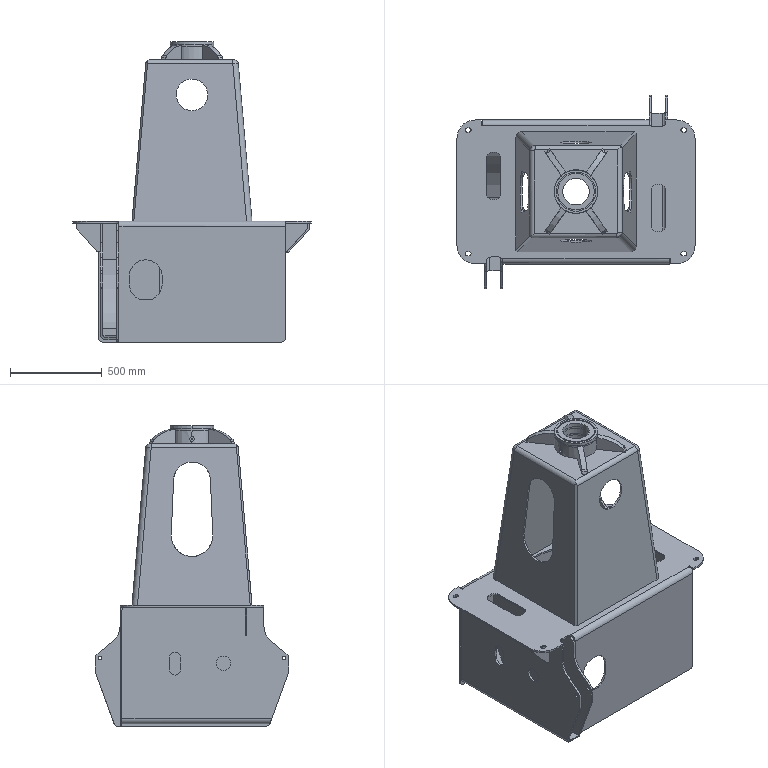Part | SolidWorks | features DeleteBody 3, MBimport 1 | 25 solids | 441 faces | box 1300 x 1057 x 1641 mm | volume 81137249 mm3 | plane 233 | cylinder 201 | spline 5 | cone 2 | commonest cylinder face diameters 40 x21 80 x14 23 x12 50 x11 30 x9 20.686 x8